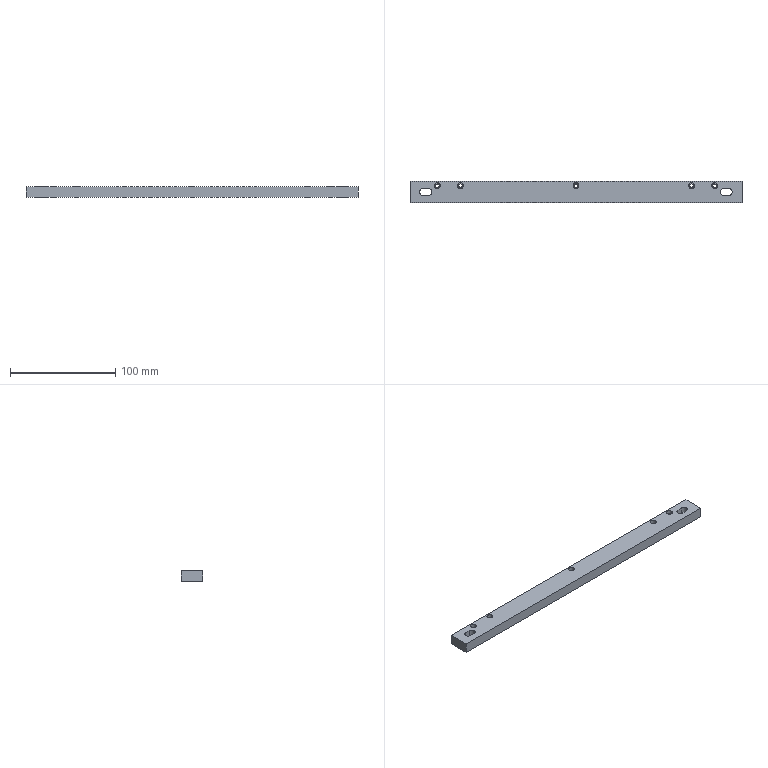Part | STEP file | CA-10-005Lift Stop Plate1_Default | 1 solid | 41 faces | box 316 x 20 x 10 mm | volume 61183 mm3 | cylinder 26 | plane 15 | commonest cylinder face diameters 3.4 x10 5.5 x10 6.5 x6